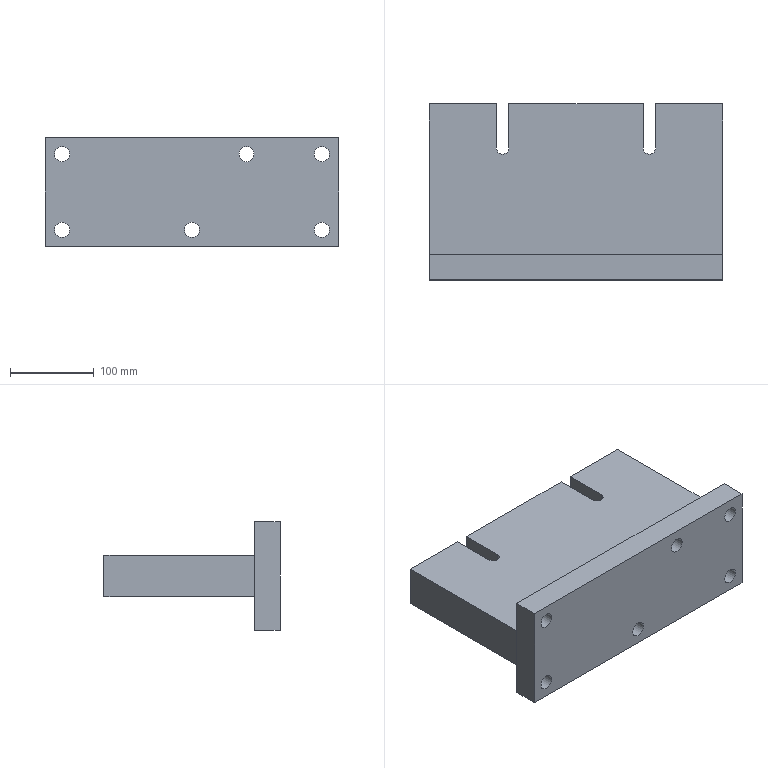Part | NX | features lower clamp stand 3 | 2 solids | 26 faces | box 350 x 210 x 130 mm | volume 4381610 mm3 | plane 18 | cylinder 8 | commonest cylinder face diameters 18 x6 15 x2
STEP:
#1=CARTESIAN_POINT('',(175.,-180.,-36.));
#2=VERTEX_POINT('',#1);
#3=CARTESIAN_POINT('',(175.,-180.,-45.));
#4=DIRECTION('',(0.,1.,0.));
#5=DIRECTION('',(0.,0.,1.));
#6=AXIS2_PLACEMENT_3D('',#3,#4,#5);
#7=CIRCLE('',#6,9.);
#8=EDGE_CURVE('',#2,#2,#7,.F.);
#9=ORIENTED_EDGE('',*,*,#8,.T.);
#10=EDGE_LOOP('',(#9));
#11=FACE_BOUND('',#10,.T.);
#12=CARTESIAN_POINT('',(20.,-180.,54.));
#13=VERTEX_POINT('',#12);
#14=CARTESIAN_POINT('',(20.,-180.,45.));
#15=DIRECTION('',(0.,1.,0.));
#16=DIRECTION('',(0.,0.,1.));
#17=AXIS2_PLACEMENT_3D('',#14,#15,#16);
#18=CIRCLE('',#17,9.);
#19=EDGE_CURVE('',#13,#13,#18,.F.);
#20=ORIENTED_EDGE('',*,*,#19,.T.);
#21=EDGE_LOOP('',(#20));
#22=FACE_BOUND('',#21,.T.);
#23=CARTESIAN_POINT('',(330.,-180.,-36.));
#24=VERTEX_POINT('',#23);
#25=CARTESIAN_POINT('',(330.,-180.,-45.));
#26=DIRECTION('',(0.,1.,0.));
#27=DIRECTION('',(0.,0.,1.));
#28=AXIS2_PLACEMENT_3D('',#25,#26,#27);
#29=CIRCLE('',#28,9.);
#30=EDGE_CURVE('',#24,#24,#29,.F.);
#31=ORIENTED_EDGE('',*,*,#30,.T.);
#32=EDGE_LOOP('',(#31));
#33=FACE_BOUND('',#32,.T.);
#34=CARTESIAN_POINT('',(0.,-180.,-65.));
#35=VERTEX_POINT('',#34);
#36=CARTESIAN_POINT('',(0.,-180.,65.));
#37=VERTEX_POINT('',#36);
#38=CARTESIAN_POINT('',(0.,-180.,-65.));
#39=DIRECTION('',(0.,0.,-1.));
#40=VECTOR('',#39,1000.);
#41=LINE('',#38,#40);
#42=EDGE_CURVE('',#35,#37,#41,.F.);
#43=ORIENTED_EDGE('',*,*,#42,.T.);
#44=CARTESIAN_POINT('',(350.,-180.,65.));
#45=VERTEX_POINT('',#44);
#46=CARTESIAN_POINT('',(0.,-180.,65.));
#47=DIRECTION('',(-1.,0.,0.));
#48=VECTOR('',#47,1000.);
#49=LINE('',#46,#48);
#50=EDGE_CURVE('',#37,#45,#49,.F.);
#51=ORIENTED_EDGE('',*,*,#50,.T.);
#52=CARTESIAN_POINT('',(350.,-180.,-65.));
#53=VERTEX_POINT('',#52);
#54=CARTESIAN_POINT('',(350.,-180.,-65.));
#55=DIRECTION('',(0.,0.,1.));
#56=VECTOR('',#55,1000.);
#57=LINE('',#54,#56);
#58=EDGE_CURVE('',#45,#53,#57,.F.);
#59=ORIENTED_EDGE('',*,*,#58,.T.);
#60=CARTESIAN_POINT('',(0.,-180.,-65.));
#61=DIRECTION('',(1.,0.,0.));
#62=VECTOR('',#61,1000.);
#63=LINE('',#60,#62);
#64=EDGE_CURVE('',#53,#35,#63,.F.);
#65=ORIENTED_EDGE('',*,*,#64,.T.);
#66=EDGE_LOOP('',(#43,#51,#59,#65));
#67=FACE_BOUND('',#66,.T.);
#68=CARTESIAN_POINT('',(330.,-180.,54.));
#69=VERTEX_POINT('',#68);
#70=CARTESIAN_POINT('',(330.,-180.,45.));
#71=DIRECTION('',(0.,1.,0.));
#72=DIRECTION('',(0.,0.,1.));
#73=AXIS2_PLACEMENT_3D('',#70,#71,#72);
#74=CIRCLE('',#73,9.);
#75=EDGE_CURVE('',#69,#69,#74,.F.);
#76=ORIENTED_EDGE('',*,*,#75,.T.);
#77=EDGE_LOOP('',(#76));
#78=FACE_BOUND('',#77,.T.);
#79=CARTESIAN_POINT('',(20.,-180.,-36.));
#80=VERTEX_POINT('',#79);
#81=CARTESIAN_POINT('',(20.,-180.,-45.));
#82=DIRECTION('',(0.,1.,0.));
#83=DIRECTION('',(0.,0.,1.));
#84=AXIS2_PLACEMENT_3D('',#81,#82,#83);
#85=CIRCLE('',#84,9.);
#86=EDGE_CURVE('',#80,#80,#85,.F.);
#87=ORIENTED_EDGE('',*,*,#86,.T.);
#88=EDGE_LOOP('',(#87));
#89=FACE_BOUND('',#88,.T.);
#90=CARTESIAN_POINT('',(240.,-180.,54.));
#91=VERTEX_POINT('',#90);
#92=CARTESIAN_POINT('',(240.,-180.,45.));
#93=DIRECTION('',(0.,1.,0.));
#94=DIRECTION('',(0.,0.,1.));
#95=AXIS2_PLACEMENT_3D('',#92,#93,#94);
#96=CIRCLE('',#95,9.);
#97=EDGE_CURVE('',#91,#91,#96,.F.);
#98=ORIENTED_EDGE('',*,*,#97,.T.);
#99=EDGE_LOOP('',(#98));
#100=FACE_BOUND('',#99,.T.);
#101=CARTESIAN_POINT('',(350.,-180.,65.));
#102=DIRECTION('',(0.,1.,0.));
#103=DIRECTION('',(0.,0.,1.));
#104=AXIS2_PLACEMENT_3D('',#101,#102,#103);
#105=PLANE('',#104);
#106=ADVANCED_FACE('',(#11,#22,#33,#67,#78,#89,#100),#105,.T.);
#107=ORIENTED_EDGE('',*,*,#97,.F.);
#108=EDGE_LOOP('',(#107));
#109=FACE_BOUND('',#108,.T.);
#110=CARTESIAN_POINT('',(240.,-210.,54.));
#111=VERTEX_POINT('',#110);
#112=CARTESIAN_POINT('',(240.,-210.,45.));
#113=DIRECTION('',(0.,1.,0.));
#114=DIRECTION('',(0.,0.,1.));
#115=AXIS2_PLACEMENT_3D('',#112,#113,#114);
#116=CIRCLE('',#115,9.);
#117=EDGE_CURVE('',#111,#111,#116,.F.);
#118=ORIENTED_EDGE('',*,*,#117,.T.);
#119=EDGE_LOOP('',(#118));
#120=FACE_BOUND('',#119,.T.);
#121=CARTESIAN_POINT('',(240.,-210.,45.));
#122=DIRECTION('',(0.,1.,0.));
#123=DIRECTION('',(0.,0.,1.));
#124=AXIS2_PLACEMENT_3D('',#121,#122,#123);
#125=CYLINDRICAL_SURFACE('',#124,9.);
#126=ADVANCED_FACE('',(#109,#120),#125,.F.);
#127=ORIENTED_EDGE('',*,*,#86,.F.);
#128=EDGE_LOOP('',(#127));
#129=FACE_BOUND('',#128,.T.);
#130=CARTESIAN_POINT('',(20.,-210.,-36.));
#131=VERTEX_POINT('',#130);
#132=CARTESIAN_POINT('',(20.,-210.,-45.));
#133=DIRECTION('',(0.,1.,0.));
#134=DIRECTION('',(0.,0.,1.));
#135=AXIS2_PLACEMENT_3D('',#132,#133,#134);
#136=CIRCLE('',#135,9.);
#137=EDGE_CURVE('',#131,#131,#136,.F.);
#138=ORIENTED_EDGE('',*,*,#137,.T.);
#139=EDGE_LOOP('',(#138));
#140=FACE_BOUND('',#139,.T.);
#141=CARTESIAN_POINT('',(20.,-210.,-45.));
#142=DIRECTION('',(0.,1.,0.));
#143=DIRECTION('',(0.,0.,1.));
#144=AXIS2_PLACEMENT_3D('',#141,#142,#143);
#145=CYLINDRICAL_SURFACE('',#144,9.);
#146=ADVANCED_FACE('',(#129,#140),#145,.F.);
#147=ORIENTED_EDGE('',*,*,#75,.F.);
#148=EDGE_LOOP('',(#147));
#149=FACE_BOUND('',#148,.T.);
#150=CARTESIAN_POINT('',(330.,-210.,54.));
#151=VERTEX_POINT('',#150);
#152=CARTESIAN_POINT('',(330.,-210.,45.));
#153=DIRECTION('',(0.,1.,0.));
#154=DIRECTION('',(0.,0.,1.));
#155=AXIS2_PLACEMENT_3D('',#152,#153,#154);
#156=CIRCLE('',#155,9.);
#157=EDGE_CURVE('',#151,#151,#156,.F.);
#158=ORIENTED_EDGE('',*,*,#157,.T.);
#159=EDGE_LOOP('',(#158));
#160=FACE_BOUND('',#159,.T.);
#161=CARTESIAN_POINT('',(330.,-210.,45.));
#162=DIRECTION('',(0.,1.,0.));
#163=DIRECTION('',(0.,0.,1.));
#164=AXIS2_PLACEMENT_3D('',#161,#162,#163);
#165=CYLINDRICAL_SURFACE('',#164,9.);
#166=ADVANCED_FACE('',(#149,#160),#165,.F.);
#167=CARTESIAN_POINT('',(350.,-210.,-65.));
#168=VERTEX_POINT('',#167);
#169=CARTESIAN_POINT('',(350.,-210.,-65.));
#170=DIRECTION('',(0.,1.,0.));
#171=VECTOR('',#170,1000.);
#172=LINE('',#169,#171);
#173=EDGE_CURVE('',#53,#168,#172,.F.);
#174=ORIENTED_EDGE('',*,*,#173,.T.);
#175=CARTESIAN_POINT('',(0.,-210.,-65.));
#176=VERTEX_POINT('',#175);
#177=CARTESIAN_POINT('',(350.,-210.,-65.));
#178=DIRECTION('',(1.,0.,0.));
#179=VECTOR('',#178,1000.);
#180=LINE('',#177,#179);
#181=EDGE_CURVE('',#168,#176,#180,.F.);
#182=ORIENTED_EDGE('',*,*,#181,.T.);
#183=CARTESIAN_POINT('',(0.,-210.,-65.));
#184=DIRECTION('',(0.,1.,0.));
#185=VECTOR('',#184,1000.);
#186=LINE('',#183,#185);
#187=EDGE_CURVE('',#176,#35,#186,.T.);
#188=ORIENTED_EDGE('',*,*,#187,.T.);
#189=ORIENTED_EDGE('',*,*,#64,.F.);
#190=EDGE_LOOP('',(#174,#182,#188,#189));
#191=FACE_BOUND('',#190,.T.);
#192=CARTESIAN_POINT('',(0.,-210.,-65.));
#193=DIRECTION('',(0.,0.,1.));
#194=DIRECTION('',(1.,0.,0.));
#195=AXIS2_PLACEMENT_3D('',#192,#193,#194);
#196=PLANE('',#195);
#197=ADVANCED_FACE('',(#191),#196,.F.);
#198=ORIENTED_EDGE('',*,*,#187,.F.);
#199=CARTESIAN_POINT('',(0.,-210.,65.));
#200=VERTEX_POINT('',#199);
#201=CARTESIAN_POINT('',(0.,-210.,65.));
#202=DIRECTION('',(0.,0.,1.));
#203=VECTOR('',#202,1000.);
#204=LINE('',#201,#203);
#205=EDGE_CURVE('',#176,#200,#204,.T.);
#206=ORIENTED_EDGE('',*,*,#205,.T.);
#207=CARTESIAN_POINT('',(0.,-210.,65.));
#208=DIRECTION('',(0.,1.,0.));
#209=VECTOR('',#208,1000.);
#210=LINE('',#207,#209);
#211=EDGE_CURVE('',#200,#37,#210,.T.);
#212=ORIENTED_EDGE('',*,*,#211,.T.);
#213=ORIENTED_EDGE('',*,*,#42,.F.);
#214=EDGE_LOOP('',(#198,#206,#212,#213));
#215=FACE_BOUND('',#214,.T.);
#216=CARTESIAN_POINT('',(0.,-210.,-65.));
#217=DIRECTION('',(1.,0.,0.));
#218=DIRECTION('',(0.,0.,-1.));
#219=AXIS2_PLACEMENT_3D('',#216,#217,#218);
#220=PLANE('',#219);
#221=ADVANCED_FACE('',(#215),#220,.F.);
#222=ORIENTED_EDGE('',*,*,#211,.F.);
#223=CARTESIAN_POINT('',(350.,-210.,65.));
#224=VERTEX_POINT('',#223);
#225=CARTESIAN_POINT('',(350.,-210.,65.));
#226=DIRECTION('',(1.,0.,0.));
#227=VECTOR('',#226,1000.);
#228=LINE('',#225,#227);
#229=EDGE_CURVE('',#200,#224,#228,.T.);
#230=ORIENTED_EDGE('',*,*,#229,.T.);
#231=CARTESIAN_POINT('',(350.,-210.,65.));
#232=DIRECTION('',(0.,1.,0.));
#233=VECTOR('',#232,1000.);
#234=LINE('',#231,#233);
#235=EDGE_CURVE('',#224,#45,#234,.T.);
#236=ORIENTED_EDGE('',*,*,#235,.T.);
#237=ORIENTED_EDGE('',*,*,#50,.F.);
#238=EDGE_LOOP('',(#222,#230,#236,#237));
#239=FACE_BOUND('',#238,.T.);
#240=CARTESIAN_POINT('',(0.,-210.,65.));
#241=DIRECTION('',(0.,0.,-1.));
#242=DIRECTION('',(-1.,0.,0.));
#243=AXIS2_PLACEMENT_3D('',#240,#241,#242);
#244=PLANE('',#243);
#245=ADVANCED_FACE('',(#239),#244,.F.);
#246=ORIENTED_EDGE('',*,*,#235,.F.);
#247=CARTESIAN_POINT('',(350.,-210.,65.));
#248=DIRECTION('',(0.,0.,1.));
#249=VECTOR('',#248,1000.);
#250=LINE('',#247,#249);
#251=EDGE_CURVE('',#224,#168,#250,.F.);
#252=ORIENTED_EDGE('',*,*,#251,.T.);
#253=ORIENTED_EDGE('',*,*,#173,.F.);
#254=ORIENTED_EDGE('',*,*,#58,.F.);
#255=EDGE_LOOP('',(#246,#252,#253,#254));
#256=FACE_BOUND('',#255,.T.);
#257=CARTESIAN_POINT('',(350.,-210.,-65.));
#258=DIRECTION('',(-1.,0.,0.));
#259=DIRECTION('',(0.,0.,1.));
#260=AXIS2_PLACEMENT_3D('',#257,#258,#259);
#261=PLANE('',#260);
#262=ADVANCED_FACE('',(#256),#261,.F.);
#263=ORIENTED_EDGE('',*,*,#30,.F.);
#264=EDGE_LOOP('',(#263));
#265=FACE_BOUND('',#264,.T.);
#266=CARTESIAN_POINT('',(330.,-210.,-36.));
#267=VERTEX_POINT('',#266);
#268=CARTESIAN_POINT('',(330.,-210.,-45.));
#269=DIRECTION('',(0.,1.,0.));
#270=DIRECTION('',(0.,0.,1.));
#271=AXIS2_PLACEMENT_3D('',#268,#269,#270);
#272=CIRCLE('',#271,9.);
#273=EDGE_CURVE('',#267,#267,#272,.F.);
#274=ORIENTED_EDGE('',*,*,#273,.T.);
#275=EDGE_LOOP('',(#274));
#276=FACE_BOUND('',#275,.T.);
#277=CARTESIAN_POINT('',(330.,-210.,-45.));
#278=DIRECTION('',(0.,1.,0.));
#279=DIRECTION('',(0.,0.,1.));
#280=AXIS2_PLACEMENT_3D('',#277,#278,#279);
#281=CYLINDRICAL_SURFACE('',#280,9.);
#282=ADVANCED_FACE('',(#265,#276),#281,.F.);
#283=ORIENTED_EDGE('',*,*,#19,.F.);
#284=EDGE_LOOP('',(#283));
#285=FACE_BOUND('',#284,.T.);
#286=CARTESIAN_POINT('',(20.,-210.,54.));
#287=VERTEX_POINT('',#286);
#288=CARTESIAN_POINT('',(20.,-210.,45.));
#289=DIRECTION('',(0.,1.,0.));
#290=DIRECTION('',(0.,0.,1.));
#291=AXIS2_PLACEMENT_3D('',#288,#289,#290);
#292=CIRCLE('',#291,9.);
#293=EDGE_CURVE('',#287,#287,#292,.F.);
#294=ORIENTED_EDGE('',*,*,#293,.T.);
#295=EDGE_LOOP('',(#294));
#296=FACE_BOUND('',#295,.T.);
#297=CARTESIAN_POINT('',(20.,-210.,45.));
#298=DIRECTION('',(0.,1.,0.));
#299=DIRECTION('',(0.,0.,1.));
#300=AXIS2_PLACEMENT_3D('',#297,#298,#299);
#301=CYLINDRICAL_SURFACE('',#300,9.);
#302=ADVANCED_FACE('',(#285,#296),#301,.F.);
#303=ORIENTED_EDGE('',*,*,#8,.F.);
#304=EDGE_LOOP('',(#303));
#305=FACE_BOUND('',#304,.T.);
#306=CARTESIAN_POINT('',(175.,-210.,-36.));
#307=VERTEX_POINT('',#306);
#308=CARTESIAN_POINT('',(175.,-210.,-45.));
#309=DIRECTION('',(0.,1.,0.));
#310=DIRECTION('',(0.,0.,1.));
#311=AXIS2_PLACEMENT_3D('',#308,#309,#310);
#312=CIRCLE('',#311,9.);
#313=EDGE_CURVE('',#307,#307,#312,.F.);
#314=ORIENTED_EDGE('',*,*,#313,.T.);
#315=EDGE_LOOP('',(#314));
#316=FACE_BOUND('',#315,.T.);
#317=CARTESIAN_POINT('',(175.,-210.,-45.));
#318=DIRECTION('',(0.,1.,0.));
#319=DIRECTION('',(0.,0.,1.));
#320=AXIS2_PLACEMENT_3D('',#317,#318,#319);
#321=CYLINDRICAL_SURFACE('',#320,9.);
#322=ADVANCED_FACE('',(#305,#316),#321,.F.);
#323=ORIENTED_EDGE('',*,*,#313,.F.);
#324=EDGE_LOOP('',(#323));
#325=FACE_BOUND('',#324,.T.);
#326=ORIENTED_EDGE('',*,*,#293,.F.);
#327=EDGE_LOOP('',(#326));
#328=FACE_BOUND('',#327,.T.);
#329=ORIENTED_EDGE('',*,*,#273,.F.);
#330=EDGE_LOOP('',(#329));
#331=FACE_BOUND('',#330,.T.);
#332=ORIENTED_EDGE('',*,*,#229,.F.);
#333=ORIENTED_EDGE('',*,*,#205,.F.);
#334=ORIENTED_EDGE('',*,*,#181,.F.);
#335=ORIENTED_EDGE('',*,*,#251,.F.);
#336=EDGE_LOOP('',(#332,#333,#334,#335));
#337=FACE_BOUND('',#336,.T.);
#338=ORIENTED_EDGE('',*,*,#157,.F.);
#339=EDGE_LOOP('',(#338));
#340=FACE_BOUND('',#339,.T.);
#341=ORIENTED_EDGE('',*,*,#137,.F.);
#342=EDGE_LOOP('',(#341));
#343=FACE_BOUND('',#342,.T.);
#344=ORIENTED_EDGE('',*,*,#117,.F.);
#345=EDGE_LOOP('',(#344));
#346=FACE_BOUND('',#345,.T.);
#347=CARTESIAN_POINT('',(350.,-210.,65.));
#348=DIRECTION('',(0.,1.,0.));
#349=DIRECTION('',(0.,0.,1.));
#350=AXIS2_PLACEMENT_3D('',#347,#348,#349);
#351=PLANE('',#350);
#352=ADVANCED_FACE('',(#325,#328,#331,#337,#340,#343,#346),#351,.F.);
#353=CLOSED_SHELL('',(#106,#126,#146,#166,#197,#221,#245,#262,#282,#302,#322,#352));
#354=MANIFOLD_SOLID_BREP('',#353);
#355=CARTESIAN_POINT('',(255.,-52.5,25.));
#356=VERTEX_POINT('',#355);
#357=CARTESIAN_POINT('',(255.,0.,25.));
#358=VERTEX_POINT('',#357);
#359=CARTESIAN_POINT('',(255.,0.,25.));
#360=DIRECTION('',(0.,1.,0.));
#361=VECTOR('',#360,1000.);
#362=LINE('',#359,#361);
#363=EDGE_CURVE('',#356,#358,#362,.T.);
#364=ORIENTED_EDGE('',*,*,#363,.T.);
#365=CARTESIAN_POINT('',(95.,0.,25.));
#366=VERTEX_POINT('',#365);
#367=CARTESIAN_POINT('',(0.,0.,25.));
#368=DIRECTION('',(1.,0.,0.));
#369=VECTOR('',#368,1000.);
#370=LINE('',#367,#369);
#371=EDGE_CURVE('',#358,#366,#370,.F.);
#372=ORIENTED_EDGE('',*,*,#371,.T.);
#373=CARTESIAN_POINT('',(95.,-52.5,25.));
#374=VERTEX_POINT('',#373);
#375=CARTESIAN_POINT('',(95.,0.,25.));
#376=DIRECTION('',(0.,1.,0.));
#377=VECTOR('',#376,1000.);
#378=LINE('',#375,#377);
#379=EDGE_CURVE('',#366,#374,#378,.F.);
#380=ORIENTED_EDGE('',*,*,#379,.T.);
#381=CARTESIAN_POINT('',(80.,-52.5,25.));
#382=VERTEX_POINT('',#381);
#383=CARTESIAN_POINT('',(87.5,-52.5,25.));
#384=DIRECTION('',(0.,0.,-1.));
#385=DIRECTION('',(-1.,0.,0.));
#386=AXIS2_PLACEMENT_3D('',#383,#384,#385);
#387=CIRCLE('',#386,7.5);
#388=EDGE_CURVE('',#374,#382,#387,.T.);
#389=ORIENTED_EDGE('',*,*,#388,.T.);
#390=CARTESIAN_POINT('',(80.,0.,25.));
#391=VERTEX_POINT('',#390);
#392=CARTESIAN_POINT('',(80.,0.,25.));
#393=DIRECTION('',(0.,1.,0.));
#394=VECTOR('',#393,1000.);
#395=LINE('',#392,#394);
#396=EDGE_CURVE('',#382,#391,#395,.T.);
#397=ORIENTED_EDGE('',*,*,#396,.T.);
#398=CARTESIAN_POINT('',(0.,0.,25.));
#399=VERTEX_POINT('',#398);
#400=CARTESIAN_POINT('',(0.,0.,25.));
#401=DIRECTION('',(1.,0.,0.));
#402=VECTOR('',#401,1000.);
#403=LINE('',#400,#402);
#404=EDGE_CURVE('',#391,#399,#403,.F.);
#405=ORIENTED_EDGE('',*,*,#404,.T.);
#406=CARTESIAN_POINT('',(0.,-180.,25.));
#407=VERTEX_POINT('',#406);
#408=CARTESIAN_POINT('',(0.,0.,25.));
#409=DIRECTION('',(0.,1.,0.));
#410=VECTOR('',#409,1000.);
#411=LINE('',#408,#410);
#412=EDGE_CURVE('',#399,#407,#411,.F.);
#413=ORIENTED_EDGE('',*,*,#412,.T.);
#414=CARTESIAN_POINT('',(350.,-180.,25.));
#415=VERTEX_POINT('',#414);
#416=CARTESIAN_POINT('',(0.,-180.,25.));
#417=DIRECTION('',(1.,0.,0.));
#418=VECTOR('',#417,1000.);
#419=LINE('',#416,#418);
#420=EDGE_CURVE('',#407,#415,#419,.T.);
#421=ORIENTED_EDGE('',*,*,#420,.T.);
#422=CARTESIAN_POINT('',(350.,0.,25.));
#423=VERTEX_POINT('',#422);
#424=CARTESIAN_POINT('',(350.,0.,25.));
#425=DIRECTION('',(0.,1.,0.));
#426=VECTOR('',#425,1000.);
#427=LINE('',#424,#426);
#428=EDGE_CURVE('',#415,#423,#427,.T.);
#429=ORIENTED_EDGE('',*,*,#428,.T.);
#430=CARTESIAN_POINT('',(270.,0.,25.));
#431=VERTEX_POINT('',#430);
#432=CARTESIAN_POINT('',(0.,0.,25.));
#433=DIRECTION('',(1.,0.,0.));
#434=VECTOR('',#433,1000.);
#435=LINE('',#432,#434);
#436=EDGE_CURVE('',#423,#431,#435,.F.);
#437=ORIENTED_EDGE('',*,*,#436,.T.);
#438=CARTESIAN_POINT('',(270.,-52.5,25.));
#439=VERTEX_POINT('',#438);
#440=CARTESIAN_POINT('',(270.,0.,25.));
#441=DIRECTION('',(0.,1.,0.));
#442=VECTOR('',#441,1000.);
#443=LINE('',#440,#442);
#444=EDGE_CURVE('',#431,#439,#443,.F.);
#445=ORIENTED_EDGE('',*,*,#444,.T.);
#446=CARTESIAN_POINT('',(262.5,-52.5,25.));
#447=DIRECTION('',(0.,0.,-1.));
#448=DIRECTION('',(-1.,0.,0.));
#449=AXIS2_PLACEMENT_3D('',#446,#447,#448);
#450=CIRCLE('',#449,7.5);
#451=EDGE_CURVE('',#439,#356,#450,.T.);
#452=ORIENTED_EDGE('',*,*,#451,.T.);
#453=EDGE_LOOP('',(#364,#372,#380,#389,#397,#405,#413,#421,#429,#437,#445,#452));
#454=FACE_BOUND('',#453,.T.);
#455=CARTESIAN_POINT('',(0.,-180.,25.));
#456=DIRECTION('',(0.,0.,1.));
#457=DIRECTION('',(1.,0.,0.));
#458=AXIS2_PLACEMENT_3D('',#455,#456,#457);
#459=PLANE('',#458);
#460=ADVANCED_FACE('',(#454),#459,.T.);
#461=CARTESIAN_POINT('',(80.,-52.5,-25.));
#462=VERTEX_POINT('',#461);
#463=CARTESIAN_POINT('',(80.,-52.5,25.));
#464=DIRECTION('',(0.,0.,-1.));
#465=VECTOR('',#464,1000.);
#466=LINE('',#463,#465);
#467=EDGE_CURVE('',#382,#462,#466,.T.);
#468=ORIENTED_EDGE('',*,*,#467,.T.);
#469=CARTESIAN_POINT('',(80.,0.,-25.));
#470=VERTEX_POINT('',#469);
#471=CARTESIAN_POINT('',(80.,-180.,-25.));
#472=DIRECTION('',(0.,1.,0.));
#473=VECTOR('',#472,1000.);
#474=LINE('',#471,#473);
#475=EDGE_CURVE('',#462,#470,#474,.T.);
#476=ORIENTED_EDGE('',*,*,#475,.T.);
#477=CARTESIAN_POINT('',(80.,0.,25.));
#478=DIRECTION('',(0.,0.,-1.));
#479=VECTOR('',#478,1000.);
#480=LINE('',#477,#479);
#481=EDGE_CURVE('',#470,#391,#480,.F.);
#482=ORIENTED_EDGE('',*,*,#481,.T.);
#483=ORIENTED_EDGE('',*,*,#396,.F.);
#484=EDGE_LOOP('',(#468,#476,#482,#483));
#485=FACE_BOUND('',#484,.T.);
#486=CARTESIAN_POINT('',(80.,0.,65.));
#487=DIRECTION('',(-1.,0.,0.));
#488=DIRECTION('',(0.,0.,1.));
#489=AXIS2_PLACEMENT_3D('',#486,#487,#488);
#490=PLANE('',#489);
#491=ADVANCED_FACE('',(#485),#490,.F.);
#492=ORIENTED_EDGE('',*,*,#481,.F.);
#493=CARTESIAN_POINT('',(0.,0.,-25.));
#494=VERTEX_POINT('',#493);
#495=CARTESIAN_POINT('',(0.,0.,-25.));
#496=DIRECTION('',(1.,0.,0.));
#497=VECTOR('',#496,1000.);
#498=LINE('',#495,#497);
#499=EDGE_CURVE('',#470,#494,#498,.F.);
#500=ORIENTED_EDGE('',*,*,#499,.T.);
#501=CARTESIAN_POINT('',(0.,0.,25.));
#502=DIRECTION('',(0.,0.,1.));
#503=VECTOR('',#502,1000.);
#504=LINE('',#501,#503);
#505=EDGE_CURVE('',#494,#399,#504,.T.);
#506=ORIENTED_EDGE('',*,*,#505,.T.);
#507=ORIENTED_EDGE('',*,*,#404,.F.);
#508=EDGE_LOOP('',(#492,#500,#506,#507));
#509=FACE_BOUND('',#508,.T.);
#510=CARTESIAN_POINT('',(0.,0.,25.));
#511=DIRECTION('',(0.,-1.,0.));
#512=DIRECTION('',(0.,0.,-1.));
#513=AXIS2_PLACEMENT_3D('',#510,#511,#512);
#514=PLANE('',#513);
#515=ADVANCED_FACE('',(#509),#514,.F.);
#516=CARTESIAN_POINT('',(0.,-180.,-25.));
#517=VERTEX_POINT('',#516);
#518=CARTESIAN_POINT('',(0.,-180.,25.));
#519=DIRECTION('',(0.,0.,1.));
#520=VECTOR('',#519,1000.);
#521=LINE('',#518,#520);
#522=EDGE_CURVE('',#517,#407,#521,.T.);
#523=ORIENTED_EDGE('',*,*,#522,.T.);
#524=ORIENTED_EDGE('',*,*,#412,.F.);
#525=ORIENTED_EDGE('',*,*,#505,.F.);
#526=CARTESIAN_POINT('',(0.,-180.,-25.));
#527=DIRECTION('',(0.,1.,0.));
#528=VECTOR('',#527,1000.);
#529=LINE('',#526,#528);
#530=EDGE_CURVE('',#494,#517,#529,.F.);
#531=ORIENTED_EDGE('',*,*,#530,.T.);
#532=EDGE_LOOP('',(#523,#524,#525,#531));
#533=FACE_BOUND('',#532,.T.);
#534=CARTESIAN_POINT('',(0.,0.,25.));
#535=DIRECTION('',(1.,0.,0.));
#536=DIRECTION('',(0.,1.,0.));
#537=AXIS2_PLACEMENT_3D('',#534,#535,#536);
#538=PLANE('',#537);
#539=ADVANCED_FACE('',(#533),#538,.F.);
#540=CARTESIAN_POINT('',(350.,-180.,-25.));
#541=VERTEX_POINT('',#540);
#542=CARTESIAN_POINT('',(350.,-180.,25.));
#543=DIRECTION('',(0.,0.,1.));
#544=VECTOR('',#543,1000.);
#545=LINE('',#542,#544);
#546=EDGE_CURVE('',#541,#415,#545,.T.);
#547=ORIENTED_EDGE('',*,*,#546,.T.);
#548=ORIENTED_EDGE('',*,*,#420,.F.);
#549=ORIENTED_EDGE('',*,*,#522,.F.);
#550=CARTESIAN_POINT('',(0.,-180.,-25.));
#551=DIRECTION('',(1.,0.,0.));
#552=VECTOR('',#551,1000.);
#553=LINE('',#550,#552);
#554=EDGE_CURVE('',#517,#541,#553,.T.);
#555=ORIENTED_EDGE('',*,*,#554,.T.);
#556=EDGE_LOOP('',(#547,#548,#549,#555));
#557=FACE_BOUND('',#556,.T.);
#558=CARTESIAN_POINT('',(0.,-180.,25.));
#559=DIRECTION('',(0.,1.,0.));
#560=DIRECTION('',(0.,0.,1.));
#561=AXIS2_PLACEMENT_3D('',#558,#559,#560);
#562=PLANE('',#561);
#563=ADVANCED_FACE('',(#557),#562,.F.);
#564=CARTESIAN_POINT('',(350.,0.,-25.));
#565=VERTEX_POINT('',#564);
#566=CARTESIAN_POINT('',(350.,0.,25.));
#567=DIRECTION('',(0.,0.,-1.));
#568=VECTOR('',#567,1000.);
#569=LINE('',#566,#568);
#570=EDGE_CURVE('',#565,#423,#569,.F.);
#571=ORIENTED_EDGE('',*,*,#570,.T.);
#572=ORIENTED_EDGE('',*,*,#428,.F.);
#573=ORIENTED_EDGE('',*,*,#546,.F.);
#574=CARTESIAN_POINT('',(350.,-180.,-25.));
#575=DIRECTION('',(0.,1.,0.));
#576=VECTOR('',#575,1000.);
#577=LINE('',#574,#576);
#578=EDGE_CURVE('',#541,#565,#577,.T.);
#579=ORIENTED_EDGE('',*,*,#578,.T.);
#580=EDGE_LOOP('',(#571,#572,#573,#579));
#581=FACE_BOUND('',#580,.T.);
#582=CARTESIAN_POINT('',(350.,0.,25.));
#583=DIRECTION('',(-1.,0.,0.));
#584=DIRECTION('',(0.,0.,1.));
#585=AXIS2_PLACEMENT_3D('',#582,#583,#584);
#586=PLANE('',#585);
#587=ADVANCED_FACE('',(#581),#586,.F.);
#588=CARTESIAN_POINT('',(270.,0.,-25.));
#589=VERTEX_POINT('',#588);
#590=CARTESIAN_POINT('',(270.,0.,65.));
#591=DIRECTION('',(0.,0.,-1.));
#592=VECTOR('',#591,1000.);
#593=LINE('',#590,#592);
#594=EDGE_CURVE('',#589,#431,#593,.F.);
#595=ORIENTED_EDGE('',*,*,#594,.T.);
#596=ORIENTED_EDGE('',*,*,#436,.F.);
#597=ORIENTED_EDGE('',*,*,#570,.F.);
#598=CARTESIAN_POINT('',(0.,0.,-25.));
#599=DIRECTION('',(1.,0.,0.));
#600=VECTOR('',#599,1000.);
#601=LINE('',#598,#600);
#602=EDGE_CURVE('',#565,#589,#601,.F.);
#603=ORIENTED_EDGE('',*,*,#602,.T.);
#604=EDGE_LOOP('',(#595,#596,#597,#603));
#605=FACE_BOUND('',#604,.T.);
#606=CARTESIAN_POINT('',(0.,0.,25.));
#607=DIRECTION('',(0.,-1.,0.));
#608=DIRECTION('',(0.,0.,-1.));
#609=AXIS2_PLACEMENT_3D('',#606,#607,#608);
#610=PLANE('',#609);
#611=ADVANCED_FACE('',(#605),#610,.F.);
#612=CARTESIAN_POINT('',(270.,-52.5,-25.));
#613=VERTEX_POINT('',#612);
#614=CARTESIAN_POINT('',(270.,-52.5,-25.));
#615=DIRECTION('',(0.,0.,-1.));
#616=VECTOR('',#615,1000.);
#617=LINE('',#614,#616);
#618=EDGE_CURVE('',#613,#439,#617,.F.);
#619=ORIENTED_EDGE('',*,*,#618,.T.);
#620=ORIENTED_EDGE('',*,*,#444,.F.);
#621=ORIENTED_EDGE('',*,*,#594,.F.);
#622=CARTESIAN_POINT('',(270.,-180.,-25.));
#623=DIRECTION('',(0.,1.,0.));
#624=VECTOR('',#623,1000.);
#625=LINE('',#622,#624);
#626=EDGE_CURVE('',#589,#613,#625,.F.);
#627=ORIENTED_EDGE('',*,*,#626,.T.);
#628=EDGE_LOOP('',(#619,#620,#621,#627));
#629=FACE_BOUND('',#628,.T.);
#630=CARTESIAN_POINT('',(270.,0.,65.));
#631=DIRECTION('',(1.,0.,0.));
#632=DIRECTION('',(0.,0.,-1.));
#633=AXIS2_PLACEMENT_3D('',#630,#631,#632);
#634=PLANE('',#633);
#635=ADVANCED_FACE('',(#629),#634,.F.);
#636=CARTESIAN_POINT('',(255.,-52.5,-25.));
#637=VERTEX_POINT('',#636);
#638=CARTESIAN_POINT('',(262.5,-52.5,-25.));
#639=DIRECTION('',(0.,0.,-1.));
#640=DIRECTION('',(-1.,0.,0.));
#641=AXIS2_PLACEMENT_3D('',#638,#639,#640);
#642=CIRCLE('',#641,7.5);
#643=EDGE_CURVE('',#613,#637,#642,.T.);
#644=ORIENTED_EDGE('',*,*,#643,.T.);
#645=CARTESIAN_POINT('',(255.,-52.5,65.));
#646=DIRECTION('',(0.,0.,1.));
#647=VECTOR('',#646,1000.);
#648=LINE('',#645,#647);
#649=EDGE_CURVE('',#637,#356,#648,.T.);
#650=ORIENTED_EDGE('',*,*,#649,.T.);
#651=ORIENTED_EDGE('',*,*,#451,.F.);
#652=ORIENTED_EDGE('',*,*,#618,.F.);
#653=EDGE_LOOP('',(#644,#650,#651,#652));
#654=FACE_BOUND('',#653,.T.);
#655=CARTESIAN_POINT('',(262.5,-52.5,-25.));
#656=DIRECTION('',(0.,0.,-1.));
#657=DIRECTION('',(-1.,0.,0.));
#658=AXIS2_PLACEMENT_3D('',#655,#656,#657);
#659=CYLINDRICAL_SURFACE('',#658,7.5);
#660=ADVANCED_FACE('',(#654),#659,.F.);
#661=ORIENTED_EDGE('',*,*,#649,.F.);
#662=CARTESIAN_POINT('',(255.,0.,-25.));
#663=VERTEX_POINT('',#662);
#664=CARTESIAN_POINT('',(255.,-180.,-25.));
#665=DIRECTION('',(0.,1.,0.));
#666=VECTOR('',#665,1000.);
#667=LINE('',#664,#666);
#668=EDGE_CURVE('',#637,#663,#667,.T.);
#669=ORIENTED_EDGE('',*,*,#668,.T.);
#670=CARTESIAN_POINT('',(255.,0.,25.));
#671=DIRECTION('',(0.,0.,-1.));
#672=VECTOR('',#671,1000.);
#673=LINE('',#670,#672);
#674=EDGE_CURVE('',#663,#358,#673,.F.);
#675=ORIENTED_EDGE('',*,*,#674,.T.);
#676=ORIENTED_EDGE('',*,*,#363,.F.);
#677=EDGE_LOOP('',(#661,#669,#675,#676));
#678=FACE_BOUND('',#677,.T.);
#679=CARTESIAN_POINT('',(255.,0.,65.));
#680=DIRECTION('',(-1.,0.,0.));
#681=DIRECTION('',(0.,0.,1.));
#682=AXIS2_PLACEMENT_3D('',#679,#680,#681);
#683=PLANE('',#682);
#684=ADVANCED_FACE('',(#678),#683,.F.);
#685=CARTESIAN_POINT('',(95.,0.,-25.));
#686=VERTEX_POINT('',#685);
#687=CARTESIAN_POINT('',(95.,0.,65.));
#688=DIRECTION('',(0.,0.,1.));
#689=VECTOR('',#688,1000.);
#690=LINE('',#687,#689);
#691=EDGE_CURVE('',#686,#366,#690,.T.);
#692=ORIENTED_EDGE('',*,*,#691,.T.);
#693=ORIENTED_EDGE('',*,*,#371,.F.);
#694=ORIENTED_EDGE('',*,*,#674,.F.);
#695=CARTESIAN_POINT('',(0.,0.,-25.));
#696=DIRECTION('',(1.,0.,0.));
#697=VECTOR('',#696,1000.);
#698=LINE('',#695,#697);
#699=EDGE_CURVE('',#663,#686,#698,.F.);
#700=ORIENTED_EDGE('',*,*,#699,.T.);
#701=EDGE_LOOP('',(#692,#693,#694,#700));
#702=FACE_BOUND('',#701,.T.);
#703=CARTESIAN_POINT('',(0.,0.,25.));
#704=DIRECTION('',(0.,-1.,0.));
#705=DIRECTION('',(0.,0.,-1.));
#706=AXIS2_PLACEMENT_3D('',#703,#704,#705);
#707=PLANE('',#706);
#708=ADVANCED_FACE('',(#702),#707,.F.);
#709=CARTESIAN_POINT('',(95.,-52.5,-25.));
#710=VERTEX_POINT('',#709);
#711=CARTESIAN_POINT('',(95.,-52.5,25.));
#712=DIRECTION('',(0.,0.,-1.));
#713=VECTOR('',#712,1000.);
#714=LINE('',#711,#713);
#715=EDGE_CURVE('',#710,#374,#714,.F.);
#716=ORIENTED_EDGE('',*,*,#715,.T.);
#717=ORIENTED_EDGE('',*,*,#379,.F.);
#718=ORIENTED_EDGE('',*,*,#691,.F.);
#719=CARTESIAN_POINT('',(95.,-180.,-25.));
#720=DIRECTION('',(0.,1.,0.));
#721=VECTOR('',#720,1000.);
#722=LINE('',#719,#721);
#723=EDGE_CURVE('',#686,#710,#722,.F.);
#724=ORIENTED_EDGE('',*,*,#723,.T.);
#725=EDGE_LOOP('',(#716,#717,#718,#724));
#726=FACE_BOUND('',#725,.T.);
#727=CARTESIAN_POINT('',(95.,0.,65.));
#728=DIRECTION('',(1.,0.,0.));
#729=DIRECTION('',(0.,1.,0.));
#730=AXIS2_PLACEMENT_3D('',#727,#728,#729);
#731=PLANE('',#730);
#732=ADVANCED_FACE('',(#726),#731,.F.);
#733=ORIENTED_EDGE('',*,*,#388,.F.);
#734=ORIENTED_EDGE('',*,*,#715,.F.);
#735=CARTESIAN_POINT('',(87.5,-52.5,-25.));
#736=DIRECTION('',(0.,0.,-1.));
#737=DIRECTION('',(-1.,0.,0.));
#738=AXIS2_PLACEMENT_3D('',#735,#736,#737);
#739=CIRCLE('',#738,7.5);
#740=EDGE_CURVE('',#710,#462,#739,.T.);
#741=ORIENTED_EDGE('',*,*,#740,.T.);
#742=ORIENTED_EDGE('',*,*,#467,.F.);
#743=EDGE_LOOP('',(#733,#734,#741,#742));
#744=FACE_BOUND('',#743,.T.);
#745=CARTESIAN_POINT('',(87.5,-52.5,25.));
#746=DIRECTION('',(0.,0.,-1.));
#747=DIRECTION('',(-1.,0.,0.));
#748=AXIS2_PLACEMENT_3D('',#745,#746,#747);
#749=CYLINDRICAL_SURFACE('',#748,7.5);
#750=ADVANCED_FACE('',(#744),#749,.F.);
#751=ORIENTED_EDGE('',*,*,#723,.F.);
#752=ORIENTED_EDGE('',*,*,#699,.F.);
#753=ORIENTED_EDGE('',*,*,#668,.F.);
#754=ORIENTED_EDGE('',*,*,#643,.F.);
#755=ORIENTED_EDGE('',*,*,#626,.F.);
#756=ORIENTED_EDGE('',*,*,#602,.F.);
#757=ORIENTED_EDGE('',*,*,#578,.F.);
#758=ORIENTED_EDGE('',*,*,#554,.F.);
#759=ORIENTED_EDGE('',*,*,#530,.F.);
#760=ORIENTED_EDGE('',*,*,#499,.F.);
#761=ORIENTED_EDGE('',*,*,#475,.F.);
#762=ORIENTED_EDGE('',*,*,#740,.F.);
#763=EDGE_LOOP('',(#751,#752,#753,#754,#755,#756,#757,#758,#759,#760,#761,#762));
#764=FACE_BOUND('',#763,.T.);
#765=CARTESIAN_POINT('',(0.,-180.,-25.));
#766=DIRECTION('',(0.,0.,1.));
#767=DIRECTION('',(1.,0.,0.));
#768=AXIS2_PLACEMENT_3D('',#765,#766,#767);
#769=PLANE('',#768);
#770=ADVANCED_FACE('',(#764),#769,.F.);
#771=CLOSED_SHELL('',(#460,#491,#515,#539,#563,#587,#611,#635,#660,#684,#708,#732,#750,#770));
#772=MANIFOLD_SOLID_BREP('',#771);
#773=(LENGTH_UNIT()NAMED_UNIT(*)SI_UNIT(.MILLI.,.METRE.));
#774=UNCERTAINTY_MEASURE_WITH_UNIT(LENGTH_MEASURE(0.00001),#773,'','');
#775=(NAMED_UNIT(*)PLANE_ANGLE_UNIT()SI_UNIT($,.RADIAN.));
#776=(NAMED_UNIT(*)SI_UNIT($,.STERADIAN.)SOLID_ANGLE_UNIT());
#777=(GEOMETRIC_REPRESENTATION_CONTEXT(3)GLOBAL_UNCERTAINTY_ASSIGNED_CONTEXT((#774))GLOBAL_UNIT_ASSIGNED_CONTEXT((#773,#775,#776))REPRESENTATION_CONTEXT('',''));
#778=ADVANCED_BREP_SHAPE_REPRESENTATION('',(#354,#772),#777);